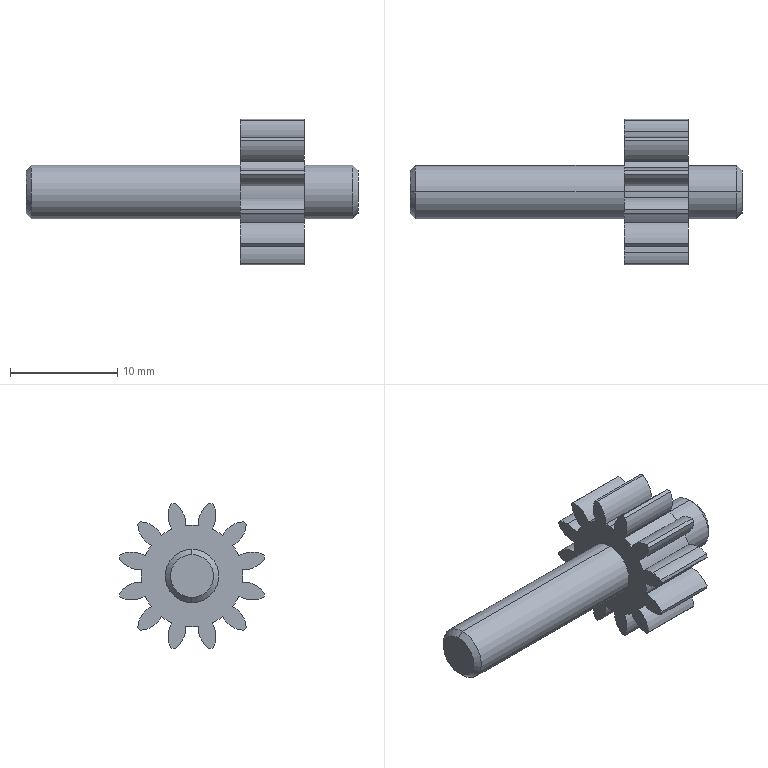Part | SolidWorks | features Boss 3, Cut 3, CirPattern 2, Fillet 2, ICE 2, Chamfer 1, Revolution 1 | 1 solid | 69 faces | box 31 x 13.609 x 13.609 mm | volume 1117 mm3 | cylinder 59 | plane 6 | cone 4 | commonest cylinder face diameters 4.8 x28 9.498 x13 14 x12 5 x4 0.8 x2